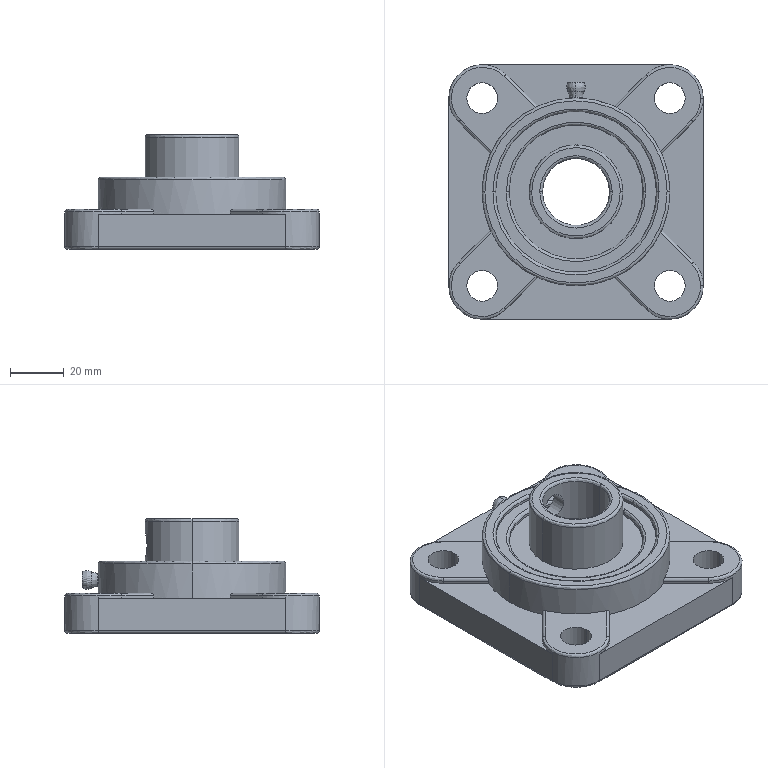Part | SolidWorks | features BaseBody 1 | 1 solid | 107 faces | box 95 x 95 x 42.9 mm | volume 150401 mm3 | cylinder 46 | spline 32 | plane 29 | commonest cylinder face diameters 2 x12 11.5 x8 25 x8 35 x4 50 x4 60 x4